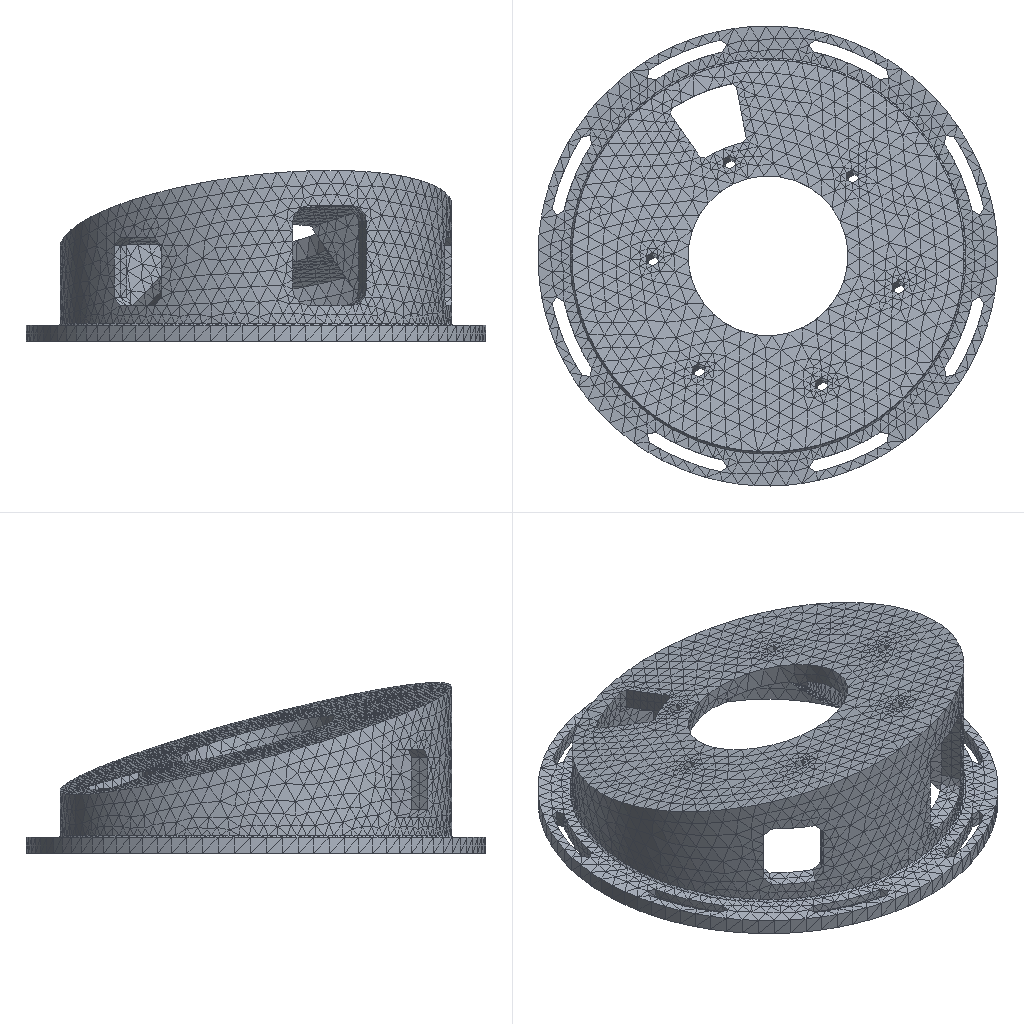Simulation study | nx simcenter
Set-up summary:
category,name,step,type,value,unit,region
solver,nx_nastran (Simcenter)
units,not stated in the deck,,not stated
analysis,deck,,static,static
analysis,solution,,SOL,101
load_step,SUBCASE 1,1,SUBCASE,SPC=1 LOAD=2
load_step,requested,,,1
mesh,nodes,,,24745
mesh,elements,,,12312
element_type,CTETRA,,solid,12312
load,nodal force total,,FX,0.0,model units
load,nodal force total,,FY,0.0,model units
load,nodal force total,,FZ,-499999.997,model units
load,load commands in deck,,count,1877
bc,support commands in deck,,count,1763
analysis,NX solution 0,,Structural,Linear Statics - Single Constraint
check,setup vs results,,match,every grid point's frame and coordinates and every element id; grid points of CTETRA elements
Nastran input file, long lists of numbers shortened:
$*$$$$$$$$$$$$$$$$$$$$$$$$$$$$$$$$$$$$$$$$$$$$$$$$$$$$$$$$$$$$$$$$$
$*
$*                    NX v10.0.0.24 TRANSLATOR
$*                    FOR NX NASTRAN VERSION 10.0
$ (33 more lines like these left out)
ASSIGN OUTPUT2='126_sim1-solution_1.op2' UNIT=12
$*
$*$$$$$$$$$$$$$$$$$$$$$$$$$$$$$$$$$$$
$*
$* EXECUTIVE CONTROL
$*
$*$$$$$$$$$$$$$$$$$$$$$$$$$$$$$$$$$$$
$*
ID,NASTRAN,126_sim1-solution_1
SOL 101
CEND
$*
$*$$$$$$$$$$$$$$$$$$$$$$$$$$$$$$$$$$$
$*
$* CASE CONTROL
$*
$*$$$$$$$$$$$$$$$$$$$$$$$$$$$$$$$$$$$
$*
TITLE = Solution 1
ECHO = NONE
SPC = 1
OUTPUT
BCRESULTS(TRACTION,FORCE,PLOT) = ALL
DISPLACEMENT(PLOT) = ALL
ESE(PLOT) = ALL
FORCE(PLOT,CORNER) = ALL
OLOAD(PLOT) = ALL
SPCFORCES(PLOT) = ALL
STRAIN(PLOT,FIBER,CORNER) = ALL
STRESS(PLOT,CORNER) = ALL
$*  NX Step: Subcase - Static Loads 1
SUBCASE 1
LABEL = Subcase - Static Loads 1
LOAD = 2
$*
$*$$$$$$$$$$$$$$$$$$$$$$$$$$$$$$$$$$$
$*
$* BULK DATA
$*
$*$$$$$$$$$$$$$$$$$$$$$$$$$$$$$$$$$$$
$*
BEGIN BULK
$*
$* PARAM CARDS
$*
PARAM      K6ROT100.0000
PARAM     OIBULK     YES
PARAM    OMACHPR     YES
PARAM       POST      -2
PARAM    POSTEXT     YES
PARAM    UNITSYS   MN-MM
$*
$* GRID CARDS
$*
GRID*              24556               0-1.078901672E+022.3873884201E+01+
*       -8.000000000E+00               0
GRID*              24557               0-1.078901672E+022.3873884201E+01+
*       0.0000000000E+00               0
$ (49486 more lines like these left out)
$*
$* ELEMENT CARDS
$*
$*  NX Mesh Collector: Solid(1)
$*  NX Mesh: 3d_mesh(1)
CTETRA         1       1   16210   16215   24094       1   16819     225+
+            226     227     228     229
CTETRA         2       1       1   24093   16206   24046     230     231+
+            232     233     234     235
$ (24620 more lines like these left out)
$*
$* PROPERTY CARDS
$*
$*  NX Property: PSOLID1
PSOLID         1       1       0                           SMECH
$*
$* MATERIAL CARDS
$*
$*  NX Material: Steel
MAT1           12.0694+8        0.2880007.8290-61.1141-5
MATT1          1       1               2               3
TABLEM1        1                                                        +
+        20.00002.0694+8 21.11002.0694+8    ENDT
TABLEM1        2                                                        +
+        20.00000.288000 21.11000.288000 23.89000.288000 37.78000.288000+
+        51.67000.289000 65.56000.289000 79.44000.290000 93.33000.290000+
+       107.22000.291000121.11000.291000135.00000.291000148.89000.292000+
+       162.78000.292000176.67000.293000190.56000.293000204.44000.293000+
+       218.33000.294000232.22000.294000246.11000.294000260.00000.295000+
+       273.89000.295000287.78000.296000301.67000.296000315.56000.296000+
+       329.44000.297000343.33000.297000357.22000.298000371.11000.298000+
+       385.00000.298000398.89000.299000412.78000.299000426.67000.300000+
+       440.56000.300000454.44000.301000468.33000.301000482.22000.302000+
+       496.11000.302000510.00000.303000523.89000.304000537.78000.304000+
+       551.67000.305000565.56000.306000579.44000.307000593.33000.308000+
+       607.22000.309000621.11000.310000635.00000.311000648.89000.312000+
+       662.78000.313000676.67000.314000690.56000.316000704.44000.317000+
+           ENDT
TABLEM1        3                                                        +
+        20.00001.1280-5 93.33001.1790-5107.22001.1880-5121.11001.1970-5+
+       135.00001.2060-5148.89001.2132-5162.78001.2222-5176.67001.2312-5+
+       190.56001.2402-5204.44001.2492-5218.33001.2582-5232.22001.2672-5+
+       246.11001.2762-5260.00001.2852-5273.89001.2942-5287.78001.3032-5+
+       301.67001.3122-5315.56001.3212-5329.44001.3302-5343.33001.3392-5+
+       357.22001.3464-5371.11001.3554-5385.00001.3644-5398.89001.3734-5+
+       412.78001.3806-5426.67001.3896-5440.56001.3986-5454.44001.4058-5+
+       468.33001.4148-5482.22001.4238-5496.11001.4310-5510.00001.4400-5+
+       523.89001.4472-5537.78001.4544-5551.67001.4616-5565.56001.4688-5+
+       579.44001.4742-5593.33001.4796-5607.22001.4832-5621.11001.4886-5+
+       635.00001.4904-5648.89001.4922-5662.78001.4922-5676.67001.4922-5+
+       690.56001.4904-5704.44001.4886-5718.33001.4850-5732.22001.4796-5+
+       746.11001.4724-5760.00001.4634-5773.89001.4472-5787.78001.4256-5+
+       801.67001.4004-5815.56001.3680-5    ENDT
$*
$* LOAD AND CONSTRAINT CARDS
$*
$*  NX Load and Constraint: Fixed(1)
SPC            1   14079  123456  0.0000
SPC            1   14080  123456  0.0000
SPC            1   14081  123456  0.0000
SPC            1   14082  123456  0.0000
$ (1759 more lines like these left out)
$*  NX Load and Constraint: Force(1)
FORCE          2   16606       0133.5846  0.0000  0.0000-1.00000
FORCE          2   16607       0155.4195  0.0000  0.0000-1.00000
FORCE          2   16608       0 84.0847  0.0000  0.0000-1.00000
FORCE          2   16609       0327.7394  0.0000  0.0000-1.00000
$ (1873 more lines like these left out)
ENDDATA 41364ae7
Results summary:
result,analysis,,,static
result,last_loadstep,,,1
result,primary field,,,displacements
result,max displacement,,,0.000304,model units
result,reaction total,,FX,-0.03384,model units
result,reaction total,,FY,-0.01029,model units
result,reaction total,,FZ,499999.781,model units
result,NX solution 0,,loadcases,1,mm